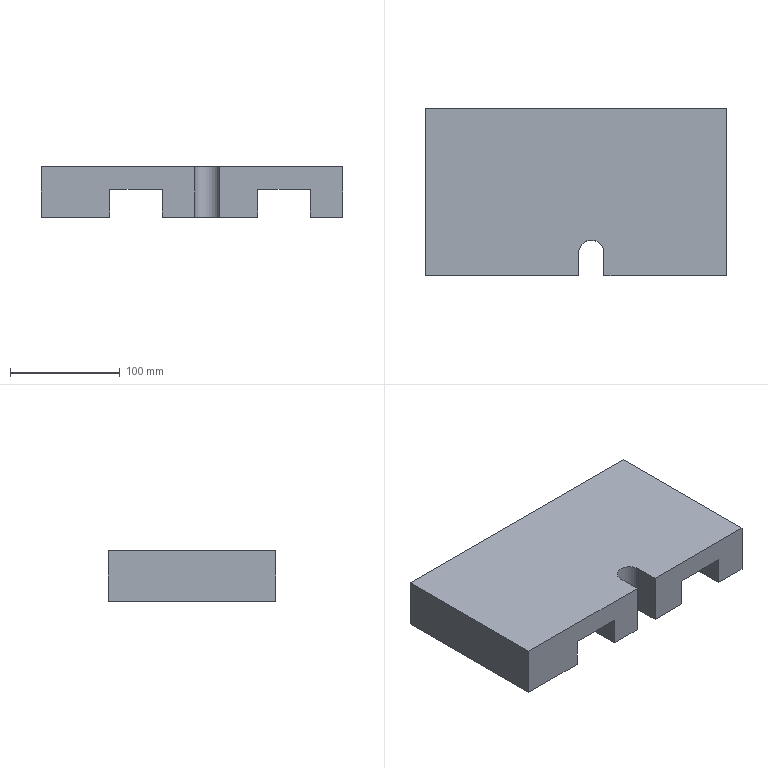Part | 1 solid | 21 faces | box 275.4 x 153 x 46 mm | volume 1522523 mm3 | plane 18 | cylinder 3 | commonest cylinder face diameters 20 x2 23 x1